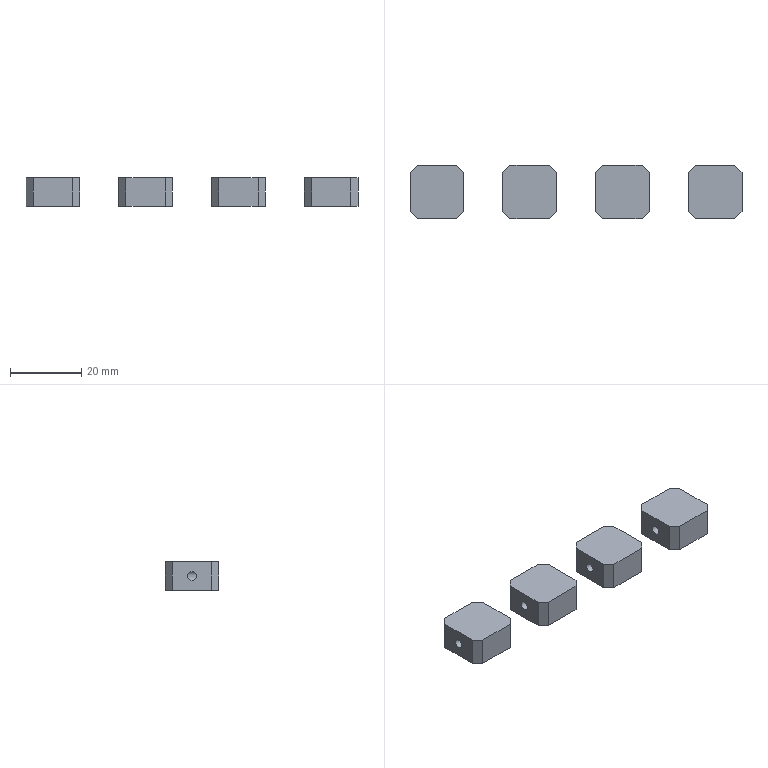CAM job | NX | 3+2 milling, drilling | part box 93 x 15 x 8 mm | stock box 98 x 20 x 10 mm
Tools:
number,name,description,diameter,corner_radius,flute_length,length,flutes
9,D10,平底铣刀-粗,10.0,0.0,35.0,75.0,2
10,D10-J,平底铣刀-精,10.0,0.0,35.0,75.0,2
1,D80R0.8飞刀,圆鼻刀-粗,80.0,0.8,50.0,75.0,2
2,D6倒角刀,倒角刀,6.0,0.0,3.0,25.0,2
21,M4X0.7,丝锥,3.3,0.0,35.0,50.0,2
13,钻头3.3,Twist Drill 3.3 mm,3.3,0.0,35.0,35.008,2
Operations:
program,operation,operation_type,tool,method,geometry_group,spindle_rpm,surface_speed,feed_per_tooth,feed_cut,feed_plunge,cut_length_mm,path_length_mm,cut_time_min,machine_time_min
A,顶面开粗,FaceMilling,D80R0.8飞刀,分层开粗-切深K-步距G,W-A,4000.0,1005.31,0.375,3000.0,100.0,187.0,222.8,0.0623,0.0659
A,顶面,FaceMilling,D80R0.8飞刀,侧刃精光-切深K-步距G,W-A,4000.0,1005.31,0.125,1000.0,100.0,187.0,223.0,0.187,0.1906
A,外形粗_2,VolumeBased25DMillingOperation,D10,METHOD,W-A,8000.0,251.327,0.3125,5000.0,80.0,10308.045,10628.545,2.062,2.094
A,等高精光往复爬面_COPY,ZLevelMilling,D10,等高爬面-切深K-步距G,W-A,7000.0,219.911,0.2857,4000.0,100.0,1312.073,1626.1,0.328,0.3594
A,打点-深0.8,Operation,D6倒角刀,NONE,W-A,8000.0,150.796,0.0312,500.0,90.0,7.2,135.458,0.0144,0.0272
A,盲锥孔-M4螺纹底孔,Operation,钻头3.3,NONE,W-A,3000.0,31.102,0.02,120.0,90.0,48.366,217.789,0.403,0.42
A,仅选体,SurfaceContour,D6倒角刀,METHOD,W-A,8000.0,150.796,0.1875,3000.0,100.0,166.525,442.766,0.0555,0.0831
A,钻倒角_1,Operation,D6倒角刀,METHOD,W-A,8000.0,150.796,0.0312,500.0,0.0,20.8,169.118,0.0416,0.0564
A,底壁铣倒角_COPY,VolumeBased25DMillingOperation,D6倒角刀,爬面_倒角-切深0-步距G,W-A,6500.0,122.519,0.1154,1500.0,100.0,156.118,464.151,0.1041,0.1349
A,盲锥孔-攻牙M4,Operation,M4X0.7,METHOD,W-A,800.0,8.294,0.0004,0.7,90.0,36.4,193.858,52.0,52.016
A,外形半精_2,VolumeBased25DMillingOperation,D10-J,METHOD,W-A,8000.0,251.327,0.0625,1000.0,100.0,667.564,1267.758,0.6676,0.7276